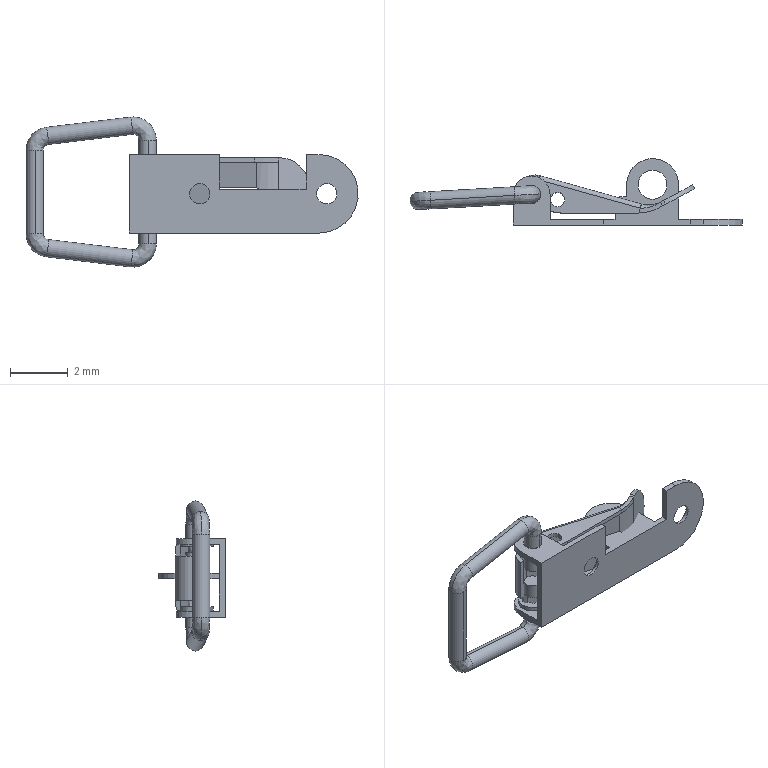Part | SolidWorks | 3 solids | 130 faces | box 11.513 x 2.3 x 5.2 mm | volume 11.366 mm3 | plane 55 | cylinder 52 | spline 19 | cone 4 | commonest cylinder face diameters 0.6 x14 0.495 x8 0.64 x4 0.7 x4 0.36 x3 1.005 x3